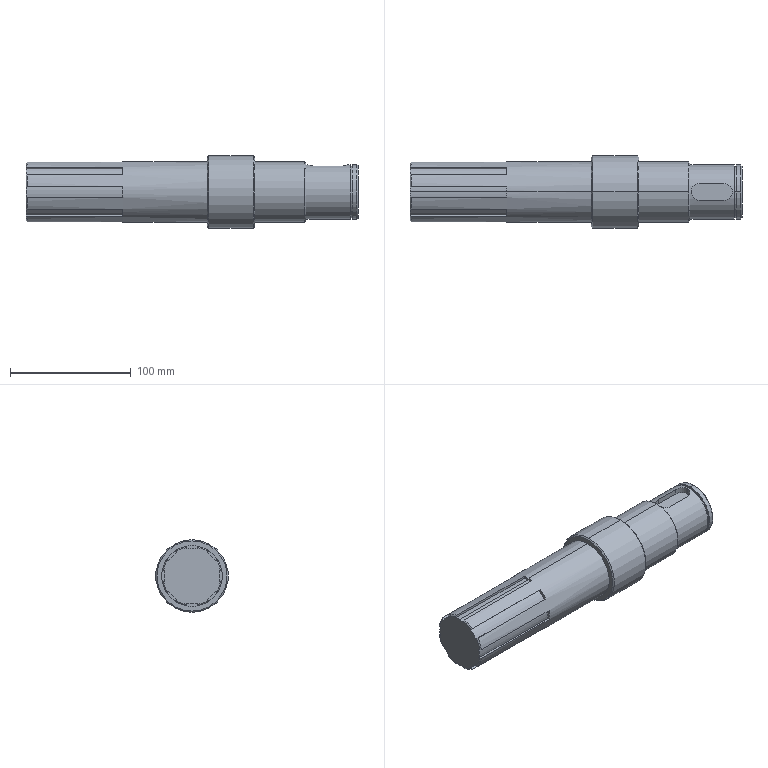Part | SolidWorks | features ICE 3, Chamfer 2, Revolution 1 | 1 solid | 74 faces | box 274.5 x 60 x 60 mm | volume 542135 mm3 | plane 34 | cylinder 24 | cone 16 | commonest cylinder face diameters 46 x9 45 x4 50 x4 14 x3 42.5 x2 60 x2